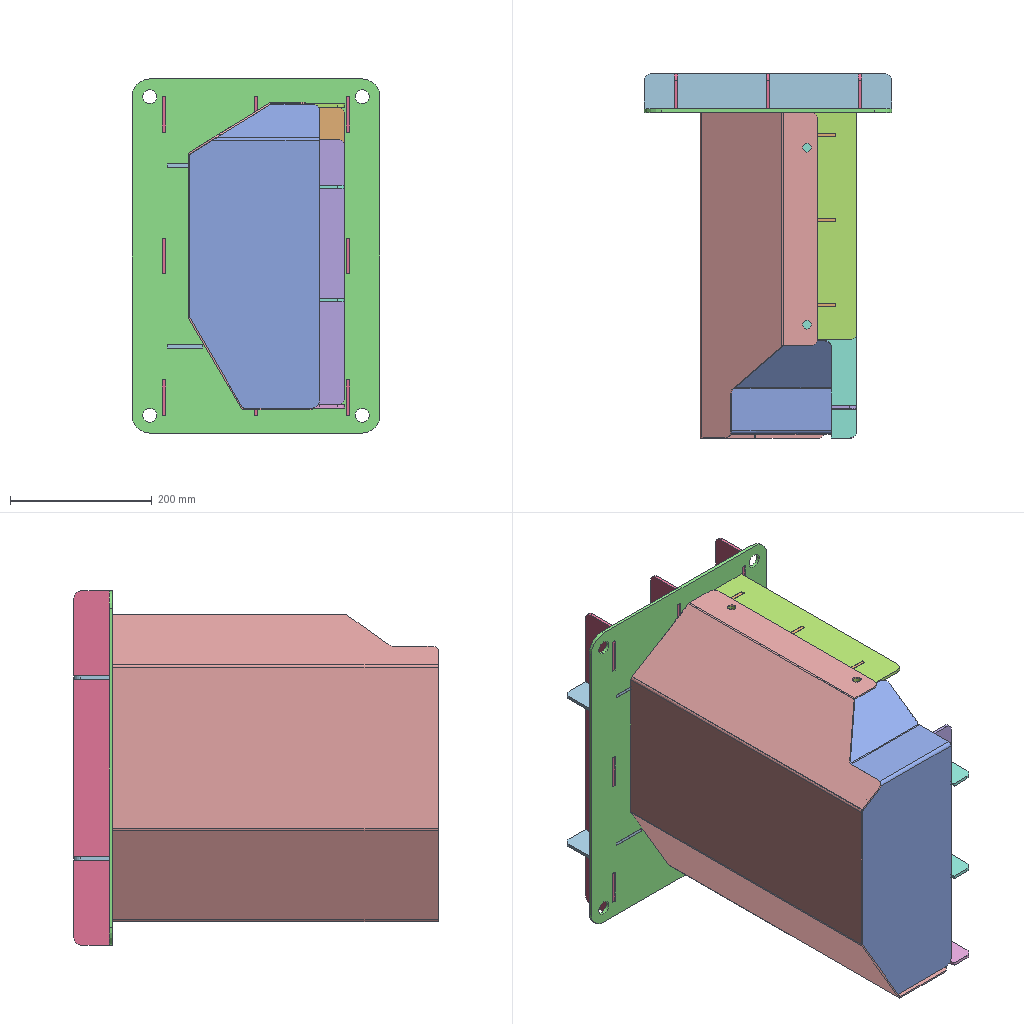Assembly | SolidWorks | 10 different items | 16 placed | box 350 x 515 x 500 mm
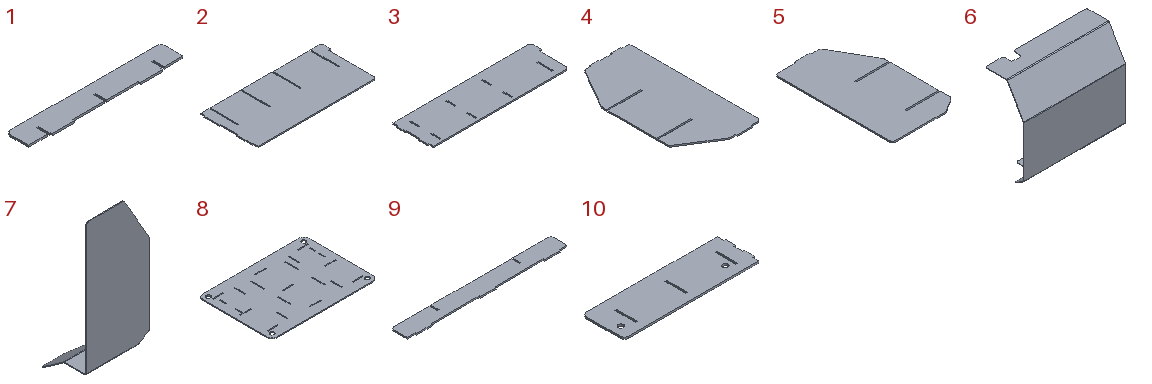Parts list (item | quantity | size | volume | features):
1 | x2 | 350 x 54 x 4.5 mm | 78838 mm3 | features FlatPattern 1, SMBaseFlange 1, SheetMetal 1
2 | x2 | 464 x 218.7 x 4.5 mm | 438971 mm3 | features Fillet 1, FlatPattern 1, SMBaseFlange 1, SheetMetal 1
3 | x1 | 464 x 135 x 4.5 mm | 271971 mm3 | features Fillet 1, FlatPattern 1, SMBaseFlange 1, SheetMetal 1
4 | x3 | 218.7 x 428.4 x 4.5 mm | 369053 mm3 | features FlatPattern 1, SMBaseFlange 1, SheetMetal 1
5 | x1 | 218.7 x 379.2 x 4.5 mm | 340357 mm3 | features FlatPattern 1, SMBaseFlange 1, SheetMetal 1
6 | x1 | 460 x 176 x 434 mm | 663913 mm3 | features ICE 3, Fillet 1, FlatPattern 1, SMBaseFlange 1, SheetMetal 1
7 | x1 | 183 x 132.321 x 429 mm | 188831 mm3 | features Fillet 2, FlatPattern 1, ICE 1, SMBaseFlange 1, SheetMetal 1
8 | x1 | 500 x 350 x 4.5 mm | 759181 mm3 | features FlatPattern 1, SMBaseFlange 1, SheetMetal 1
9 | x3 | 500 x 54 x 4.5 mm | 113974 mm3 | features FlatPattern 1, SMBaseFlange 1, SheetMetal 1
10 | x1 | 325.679 x 100 x 4.5 mm | 141321 mm3 | features Fillet 1, FlatPattern 1, SMBaseFlange 1, SheetMetal 1
Mates (type | each side: item.copy, entity, surface, feature):
DistanceDim | 7.1 face plane Base-Flange1 | 6.1 face plane Base-Flange1
Coincident | 6.1 face plane Base-Flange1 | 7.1 face plane Base-Flange1 | 2 times
InPlace | 6.1 face plane Base-Flange1 | 10.1 plane
InPlace | 6.1 face plane Base-Flange1 | 3.1 plane
InPlace | 4.1 plane | assembly plane
DistanceDim | 2.1 face plane Base-Flange1 | 3.1 face plane Base-Flange1
Coincident | 3.1 face plane Base-Flange1 | 2.1 face plane Base-Flange1 | 2 times
DistanceDim | 2.1 face plane Base-Flange1 | 2.2 face plane Base-Flange1
Coincident | 2.1 face plane Base-Flange1 | 2.2 face plane Base-Flange1 | 2 times
InPlace | 5.1 plane | assembly plane
InPlace | 6.1 face plane Base-Flange1 | 8.1 plane
InPlace | 9.1 plane | assembly plane
InPlace | 1.1 plane | assembly plane